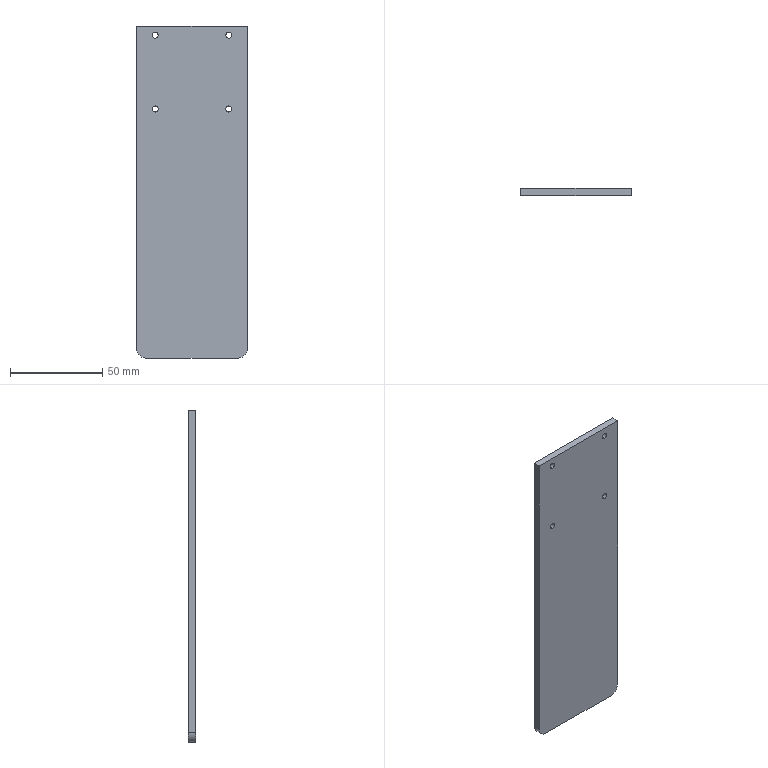Part | STEP file | PN_0021 Support plate | 1 solid | 16 faces | box 60 x 3.8 x 180 mm | volume 40869 mm3 | cylinder 10 | plane 6 | commonest cylinder face diameters 3.3 x8 10 x2
STEP:
#1=CARTESIAN_POINT('',(0.,0.,0.));
#2=DIRECTION('',(0.,0.,1.));
#3=DIRECTION('',(1.,0.,0.));
#4=AXIS2_PLACEMENT_3D('',#1,#2,#3);
#5=CARTESIAN_POINT('',(20.,0.,86.65));
#6=VERTEX_POINT('',#5);
#7=CARTESIAN_POINT('',(20.,3.8,86.65));
#8=VERTEX_POINT('',#7);
#9=CARTESIAN_POINT('',(20.,3.8,86.65));
#10=DIRECTION('',(0.,1.,0.));
#11=VECTOR('',#10,1.);
#12=LINE('',#9,#11);
#13=CARTESIAN_POINT('',(20.,3.8,85.));
#14=DIRECTION('',(0.,1.,0.));
#15=DIRECTION('',(0.,0.,1.));
#16=AXIS2_PLACEMENT_3D('',#13,#14,#15);
#17=CYLINDRICAL_SURFACE('',#16,1.65);
#18=CARTESIAN_POINT('',(6.283,0.));
#19=DIRECTION('',(0.,1.));
#20=VECTOR('',#19,1.);
#21=LINE('',#18,#20);
#22=(GEOMETRIC_REPRESENTATION_CONTEXT(2)PARAMETRIC_REPRESENTATION_CONTEXT()REPRESENTATION_CONTEXT('',''));
#23=DEFINITIONAL_REPRESENTATION('',(#21),#22);
#24=PCURVE('',#17,#23);
#25=CARTESIAN_POINT('',(20.,3.8,85.));
#26=DIRECTION('',(0.,1.,0.));
#27=DIRECTION('',(0.,0.,1.));
#28=AXIS2_PLACEMENT_3D('',#25,#26,#27);
#29=CYLINDRICAL_SURFACE('',#28,1.65);
#30=CARTESIAN_POINT('',(0.,0.));
#31=DIRECTION('',(0.,1.));
#32=VECTOR('',#31,1.);
#33=LINE('',#30,#32);
#34=(GEOMETRIC_REPRESENTATION_CONTEXT(2)PARAMETRIC_REPRESENTATION_CONTEXT()REPRESENTATION_CONTEXT('',''));
#35=DEFINITIONAL_REPRESENTATION('',(#33),#34);
#36=PCURVE('',#29,#35);
#37=SURFACE_CURVE('',#12,(#24,#36),.PCURVE_S1.);
#38=EDGE_CURVE('',#6,#8,#37,.T.);
#39=ORIENTED_EDGE('',*,*,#38,.T.);
#40=CARTESIAN_POINT('',(20.,3.8,83.35));
#41=VERTEX_POINT('',#40);
#42=CARTESIAN_POINT('',(20.,3.8,85.));
#43=DIRECTION('',(0.,-1.,0.));
#44=DIRECTION('',(0.,0.,1.));
#45=AXIS2_PLACEMENT_3D('',#42,#43,#44);
#46=CIRCLE('',#45,1.65);
#47=CARTESIAN_POINT('',(6.283,0.));
#48=DIRECTION('',(-1.,0.));
#49=VECTOR('',#48,1.);
#50=LINE('',#47,#49);
#51=(GEOMETRIC_REPRESENTATION_CONTEXT(2)PARAMETRIC_REPRESENTATION_CONTEXT()REPRESENTATION_CONTEXT('',''));
#52=DEFINITIONAL_REPRESENTATION('',(#50),#51);
#53=PCURVE('',#17,#52);
#54=CARTESIAN_POINT('',(0.,3.8,0.));
#55=DIRECTION('',(0.,1.,0.));
#56=DIRECTION('',(0.,0.,1.));
#57=AXIS2_PLACEMENT_3D('',#54,#55,#56);
#58=PLANE('',#57);
#59=CARTESIAN_POINT('',(86.65,20.));
#60=CARTESIAN_POINT('',(86.65,17.142));
#61=CARTESIAN_POINT('',(84.175,18.571));
#62=CARTESIAN_POINT('',(81.7,20.));
#63=CARTESIAN_POINT('',(84.175,21.429));
#64=CARTESIAN_POINT('',(86.65,22.858));
#65=CARTESIAN_POINT('',(86.65,20.));
#66=(BOUNDED_CURVE()B_SPLINE_CURVE(2,(#59,#60,#61,#62,#63,#64,#65),.UNSPECIFIED.,.T.,.F.)B_SPLINE_CURVE_WITH_KNOTS((1,2,2,2,2,1),(-2.094,0.,2.094,4.189,6.283,8.378),.UNSPECIFIED.)CURVE()GEOMETRIC_REPRESENTATION_ITEM()RATIONAL_B_SPLINE_CURVE((1.,0.5,1.,0.5,1.,0.5,1.))REPRESENTATION_ITEM(''));
#67=(GEOMETRIC_REPRESENTATION_CONTEXT(2)PARAMETRIC_REPRESENTATION_CONTEXT()REPRESENTATION_CONTEXT('',''));
#68=DEFINITIONAL_REPRESENTATION('',(#66),#67);
#69=PCURVE('',#58,#68);
#70=SURFACE_CURVE('',#46,(#53,#69),.PCURVE_S1.);
#71=EDGE_CURVE('',#8,#41,#70,.T.);
#72=ORIENTED_EDGE('',*,*,#71,.T.);
#73=CARTESIAN_POINT('',(20.,0.,83.35));
#74=VERTEX_POINT('',#73);
#75=CARTESIAN_POINT('',(20.,3.8,83.35));
#76=DIRECTION('',(0.,1.,0.));
#77=VECTOR('',#76,1.);
#78=LINE('',#75,#77);
#79=CARTESIAN_POINT('',(3.142,0.));
#80=DIRECTION('',(0.,1.));
#81=VECTOR('',#80,1.);
#82=LINE('',#79,#81);
#83=(GEOMETRIC_REPRESENTATION_CONTEXT(2)PARAMETRIC_REPRESENTATION_CONTEXT()REPRESENTATION_CONTEXT('',''));
#84=DEFINITIONAL_REPRESENTATION('',(#82),#83);
#85=PCURVE('',#17,#84);
#86=CARTESIAN_POINT('',(3.142,0.));
#87=DIRECTION('',(0.,1.));
#88=VECTOR('',#87,1.);
#89=LINE('',#86,#88);
#90=(GEOMETRIC_REPRESENTATION_CONTEXT(2)PARAMETRIC_REPRESENTATION_CONTEXT()REPRESENTATION_CONTEXT('',''));
#91=DEFINITIONAL_REPRESENTATION('',(#89),#90);
#92=PCURVE('',#29,#91);
#93=SURFACE_CURVE('',#78,(#85,#92),.PCURVE_S1.);
#94=EDGE_CURVE('',#74,#41,#93,.T.);
#95=ORIENTED_EDGE('',*,*,#94,.F.);
#96=CARTESIAN_POINT('',(20.,0.,85.));
#97=DIRECTION('',(0.,-1.,0.));
#98=DIRECTION('',(0.,0.,1.));
#99=AXIS2_PLACEMENT_3D('',#96,#97,#98);
#100=CIRCLE('',#99,1.65);
#101=CARTESIAN_POINT('',(6.283,-3.8));
#102=DIRECTION('',(-1.,0.));
#103=VECTOR('',#102,1.);
#104=LINE('',#101,#103);
#105=(GEOMETRIC_REPRESENTATION_CONTEXT(2)PARAMETRIC_REPRESENTATION_CONTEXT()REPRESENTATION_CONTEXT('',''));
#106=DEFINITIONAL_REPRESENTATION('',(#104),#105);
#107=PCURVE('',#17,#106);
#108=CARTESIAN_POINT('',(0.,0.,0.));
#109=DIRECTION('',(0.,1.,0.));
#110=DIRECTION('',(0.,0.,1.));
#111=AXIS2_PLACEMENT_3D('',#108,#109,#110);
#112=PLANE('',#111);
#113=CARTESIAN_POINT('',(86.65,20.));
#114=CARTESIAN_POINT('',(86.65,17.142));
#115=CARTESIAN_POINT('',(84.175,18.571));
#116=CARTESIAN_POINT('',(81.7,20.));
#117=CARTESIAN_POINT('',(84.175,21.429));
#118=CARTESIAN_POINT('',(86.65,22.858));
#119=CARTESIAN_POINT('',(86.65,20.));
#120=(BOUNDED_CURVE()B_SPLINE_CURVE(2,(#113,#114,#115,#116,#117,#118,#119),.UNSPECIFIED.,.T.,.F.)B_SPLINE_CURVE_WITH_KNOTS((1,2,2,2,2,1),(-2.094,0.,2.094,4.189,6.283,8.378),.UNSPECIFIED.)CURVE()GEOMETRIC_REPRESENTATION_ITEM()RATIONAL_B_SPLINE_CURVE((1.,0.5,1.,0.5,1.,0.5,1.))REPRESENTATION_ITEM(''));
#121=(GEOMETRIC_REPRESENTATION_CONTEXT(2)PARAMETRIC_REPRESENTATION_CONTEXT()REPRESENTATION_CONTEXT('',''));
#122=DEFINITIONAL_REPRESENTATION('',(#120),#121);
#123=PCURVE('',#112,#122);
#124=SURFACE_CURVE('',#100,(#107,#123),.PCURVE_S1.);
#125=EDGE_CURVE('',#6,#74,#124,.T.);
#126=ORIENTED_EDGE('',*,*,#125,.F.);
#127=EDGE_LOOP('',(#39,#72,#95,#126));
#128=FACE_BOUND('',#127,.F.);
#129=ADVANCED_FACE('',(#128),#17,.F.);
#130=CARTESIAN_POINT('',(20.,0.,46.65));
#131=VERTEX_POINT('',#130);
#132=CARTESIAN_POINT('',(20.,3.8,46.65));
#133=VERTEX_POINT('',#132);
#134=CARTESIAN_POINT('',(20.,3.8,46.65));
#135=DIRECTION('',(0.,1.,0.));
#136=VECTOR('',#135,1.);
#137=LINE('',#134,#136);
#138=CARTESIAN_POINT('',(20.,3.8,45.));
#139=DIRECTION('',(0.,1.,0.));
#140=DIRECTION('',(0.,0.,1.));
#141=AXIS2_PLACEMENT_3D('',#138,#139,#140);
#142=CYLINDRICAL_SURFACE('',#141,1.65);
#143=CARTESIAN_POINT('',(6.283,0.));
#144=DIRECTION('',(0.,1.));
#145=VECTOR('',#144,1.);
#146=LINE('',#143,#145);
#147=(GEOMETRIC_REPRESENTATION_CONTEXT(2)PARAMETRIC_REPRESENTATION_CONTEXT()REPRESENTATION_CONTEXT('',''));
#148=DEFINITIONAL_REPRESENTATION('',(#146),#147);
#149=PCURVE('',#142,#148);
#150=CARTESIAN_POINT('',(20.,3.8,45.));
#151=DIRECTION('',(0.,1.,0.));
#152=DIRECTION('',(0.,0.,1.));
#153=AXIS2_PLACEMENT_3D('',#150,#151,#152);
#154=CYLINDRICAL_SURFACE('',#153,1.65);
#155=CARTESIAN_POINT('',(0.,0.));
#156=DIRECTION('',(0.,1.));
#157=VECTOR('',#156,1.);
#158=LINE('',#155,#157);
#159=(GEOMETRIC_REPRESENTATION_CONTEXT(2)PARAMETRIC_REPRESENTATION_CONTEXT()REPRESENTATION_CONTEXT('',''));
#160=DEFINITIONAL_REPRESENTATION('',(#158),#159);
#161=PCURVE('',#154,#160);
#162=SURFACE_CURVE('',#137,(#149,#161),.PCURVE_S1.);
#163=EDGE_CURVE('',#131,#133,#162,.T.);
#164=ORIENTED_EDGE('',*,*,#163,.T.);
#165=CARTESIAN_POINT('',(20.,3.8,43.35));
#166=VERTEX_POINT('',#165);
#167=CARTESIAN_POINT('',(20.,3.8,45.));
#168=DIRECTION('',(0.,-1.,0.));
#169=DIRECTION('',(0.,0.,1.));
#170=AXIS2_PLACEMENT_3D('',#167,#168,#169);
#171=CIRCLE('',#170,1.65);
#172=CARTESIAN_POINT('',(6.283,0.));
#173=DIRECTION('',(-1.,0.));
#174=VECTOR('',#173,1.);
#175=LINE('',#172,#174);
#176=(GEOMETRIC_REPRESENTATION_CONTEXT(2)PARAMETRIC_REPRESENTATION_CONTEXT()REPRESENTATION_CONTEXT('',''));
#177=DEFINITIONAL_REPRESENTATION('',(#175),#176);
#178=PCURVE('',#142,#177);
#179=CARTESIAN_POINT('',(46.65,20.));
#180=CARTESIAN_POINT('',(46.65,17.142));
#181=CARTESIAN_POINT('',(44.175,18.571));
#182=CARTESIAN_POINT('',(41.7,20.));
#183=CARTESIAN_POINT('',(44.175,21.429));
#184=CARTESIAN_POINT('',(46.65,22.858));
#185=CARTESIAN_POINT('',(46.65,20.));
#186=(BOUNDED_CURVE()B_SPLINE_CURVE(2,(#179,#180,#181,#182,#183,#184,#185),.UNSPECIFIED.,.T.,.F.)B_SPLINE_CURVE_WITH_KNOTS((1,2,2,2,2,1),(-2.094,0.,2.094,4.189,6.283,8.378),.UNSPECIFIED.)CURVE()GEOMETRIC_REPRESENTATION_ITEM()RATIONAL_B_SPLINE_CURVE((1.,0.5,1.,0.5,1.,0.5,1.))REPRESENTATION_ITEM(''));
#187=(GEOMETRIC_REPRESENTATION_CONTEXT(2)PARAMETRIC_REPRESENTATION_CONTEXT()REPRESENTATION_CONTEXT('',''));
#188=DEFINITIONAL_REPRESENTATION('',(#186),#187);
#189=PCURVE('',#58,#188);
#190=SURFACE_CURVE('',#171,(#178,#189),.PCURVE_S1.);
#191=EDGE_CURVE('',#133,#166,#190,.T.);
#192=ORIENTED_EDGE('',*,*,#191,.T.);
#193=CARTESIAN_POINT('',(20.,0.,43.35));
#194=VERTEX_POINT('',#193);
#195=CARTESIAN_POINT('',(20.,3.8,43.35));
#196=DIRECTION('',(0.,1.,0.));
#197=VECTOR('',#196,1.);
#198=LINE('',#195,#197);
#199=CARTESIAN_POINT('',(3.142,0.));
#200=DIRECTION('',(0.,1.));
#201=VECTOR('',#200,1.);
#202=LINE('',#199,#201);
#203=(GEOMETRIC_REPRESENTATION_CONTEXT(2)PARAMETRIC_REPRESENTATION_CONTEXT()REPRESENTATION_CONTEXT('',''));
#204=DEFINITIONAL_REPRESENTATION('',(#202),#203);
#205=PCURVE('',#142,#204);
#206=CARTESIAN_POINT('',(3.142,0.));
#207=DIRECTION('',(0.,1.));
#208=VECTOR('',#207,1.);
#209=LINE('',#206,#208);
#210=(GEOMETRIC_REPRESENTATION_CONTEXT(2)PARAMETRIC_REPRESENTATION_CONTEXT()REPRESENTATION_CONTEXT('',''));
#211=DEFINITIONAL_REPRESENTATION('',(#209),#210);
#212=PCURVE('',#154,#211);
#213=SURFACE_CURVE('',#198,(#205,#212),.PCURVE_S1.);
#214=EDGE_CURVE('',#194,#166,#213,.T.);
#215=ORIENTED_EDGE('',*,*,#214,.F.);
#216=CARTESIAN_POINT('',(20.,0.,45.));
#217=DIRECTION('',(0.,-1.,0.));
#218=DIRECTION('',(0.,0.,1.));
#219=AXIS2_PLACEMENT_3D('',#216,#217,#218);
#220=CIRCLE('',#219,1.65);
#221=CARTESIAN_POINT('',(6.283,-3.8));
#222=DIRECTION('',(-1.,0.));
#223=VECTOR('',#222,1.);
#224=LINE('',#221,#223);
#225=(GEOMETRIC_REPRESENTATION_CONTEXT(2)PARAMETRIC_REPRESENTATION_CONTEXT()REPRESENTATION_CONTEXT('',''));
#226=DEFINITIONAL_REPRESENTATION('',(#224),#225);
#227=PCURVE('',#142,#226);
#228=CARTESIAN_POINT('',(46.65,20.));
#229=CARTESIAN_POINT('',(46.65,17.142));
#230=CARTESIAN_POINT('',(44.175,18.571));
#231=CARTESIAN_POINT('',(41.7,20.));
#232=CARTESIAN_POINT('',(44.175,21.429));
#233=CARTESIAN_POINT('',(46.65,22.858));
#234=CARTESIAN_POINT('',(46.65,20.));
#235=(BOUNDED_CURVE()B_SPLINE_CURVE(2,(#228,#229,#230,#231,#232,#233,#234),.UNSPECIFIED.,.T.,.F.)B_SPLINE_CURVE_WITH_KNOTS((1,2,2,2,2,1),(-2.094,0.,2.094,4.189,6.283,8.378),.UNSPECIFIED.)CURVE()GEOMETRIC_REPRESENTATION_ITEM()RATIONAL_B_SPLINE_CURVE((1.,0.5,1.,0.5,1.,0.5,1.))REPRESENTATION_ITEM(''));
#236=(GEOMETRIC_REPRESENTATION_CONTEXT(2)PARAMETRIC_REPRESENTATION_CONTEXT()REPRESENTATION_CONTEXT('',''));
#237=DEFINITIONAL_REPRESENTATION('',(#235),#236);
#238=PCURVE('',#112,#237);
#239=SURFACE_CURVE('',#220,(#227,#238),.PCURVE_S1.);
#240=EDGE_CURVE('',#131,#194,#239,.T.);
#241=ORIENTED_EDGE('',*,*,#240,.F.);
#242=EDGE_LOOP('',(#164,#192,#215,#241));
#243=FACE_BOUND('',#242,.F.);
#244=ADVANCED_FACE('',(#243),#142,.F.);
#245=CARTESIAN_POINT('',(-20.,0.,46.65));
#246=VERTEX_POINT('',#245);
#247=CARTESIAN_POINT('',(-20.,3.8,46.65));
#248=VERTEX_POINT('',#247);
#249=CARTESIAN_POINT('',(-20.,3.8,46.65));
#250=DIRECTION('',(0.,1.,0.));
#251=VECTOR('',#250,1.);
#252=LINE('',#249,#251);
#253=CARTESIAN_POINT('',(-20.,3.8,45.));
#254=DIRECTION('',(0.,1.,0.));
#255=DIRECTION('',(0.,0.,1.));
#256=AXIS2_PLACEMENT_3D('',#253,#254,#255);
#257=CYLINDRICAL_SURFACE('',#256,1.65);
#258=CARTESIAN_POINT('',(6.283,0.));
#259=DIRECTION('',(0.,1.));
#260=VECTOR('',#259,1.);
#261=LINE('',#258,#260);
#262=(GEOMETRIC_REPRESENTATION_CONTEXT(2)PARAMETRIC_REPRESENTATION_CONTEXT()REPRESENTATION_CONTEXT('',''));
#263=DEFINITIONAL_REPRESENTATION('',(#261),#262);
#264=PCURVE('',#257,#263);
#265=CARTESIAN_POINT('',(-20.,3.8,45.));
#266=DIRECTION('',(0.,1.,0.));
#267=DIRECTION('',(0.,0.,1.));
#268=AXIS2_PLACEMENT_3D('',#265,#266,#267);
#269=CYLINDRICAL_SURFACE('',#268,1.65);
#270=CARTESIAN_POINT('',(0.,0.));
#271=DIRECTION('',(0.,1.));
#272=VECTOR('',#271,1.);
#273=LINE('',#270,#272);
#274=(GEOMETRIC_REPRESENTATION_CONTEXT(2)PARAMETRIC_REPRESENTATION_CONTEXT()REPRESENTATION_CONTEXT('',''));
#275=DEFINITIONAL_REPRESENTATION('',(#273),#274);
#276=PCURVE('',#269,#275);
#277=SURFACE_CURVE('',#252,(#264,#276),.PCURVE_S1.);
#278=EDGE_CURVE('',#246,#248,#277,.T.);
#279=ORIENTED_EDGE('',*,*,#278,.T.);
#280=CARTESIAN_POINT('',(-20.,3.8,43.35));
#281=VERTEX_POINT('',#280);
#282=CARTESIAN_POINT('',(-20.,3.8,45.));
#283=DIRECTION('',(0.,-1.,0.));
#284=DIRECTION('',(0.,0.,1.));
#285=AXIS2_PLACEMENT_3D('',#282,#283,#284);
#286=CIRCLE('',#285,1.65);
#287=CARTESIAN_POINT('',(6.283,0.));
#288=DIRECTION('',(-1.,0.));
#289=VECTOR('',#288,1.);
#290=LINE('',#287,#289);
#291=(GEOMETRIC_REPRESENTATION_CONTEXT(2)PARAMETRIC_REPRESENTATION_CONTEXT()REPRESENTATION_CONTEXT('',''));
#292=DEFINITIONAL_REPRESENTATION('',(#290),#291);
#293=PCURVE('',#257,#292);
#294=CARTESIAN_POINT('',(46.65,-20.));
#295=CARTESIAN_POINT('',(46.65,-22.858));
#296=CARTESIAN_POINT('',(44.175,-21.429));
#297=CARTESIAN_POINT('',(41.7,-20.));
#298=CARTESIAN_POINT('',(44.175,-18.571));
#299=CARTESIAN_POINT('',(46.65,-17.142));
#300=CARTESIAN_POINT('',(46.65,-20.));
#301=(BOUNDED_CURVE()B_SPLINE_CURVE(2,(#294,#295,#296,#297,#298,#299,#300),.UNSPECIFIED.,.T.,.F.)B_SPLINE_CURVE_WITH_KNOTS((1,2,2,2,2,1),(-2.094,0.,2.094,4.189,6.283,8.378),.UNSPECIFIED.)CURVE()GEOMETRIC_REPRESENTATION_ITEM()RATIONAL_B_SPLINE_CURVE((1.,0.5,1.,0.5,1.,0.5,1.))REPRESENTATION_ITEM(''));
#302=(GEOMETRIC_REPRESENTATION_CONTEXT(2)PARAMETRIC_REPRESENTATION_CONTEXT()REPRESENTATION_CONTEXT('',''));
#303=DEFINITIONAL_REPRESENTATION('',(#301),#302);
#304=PCURVE('',#58,#303);
#305=SURFACE_CURVE('',#286,(#293,#304),.PCURVE_S1.);
#306=EDGE_CURVE('',#248,#281,#305,.T.);
#307=ORIENTED_EDGE('',*,*,#306,.T.);
#308=CARTESIAN_POINT('',(-20.,0.,43.35));
#309=VERTEX_POINT('',#308);
#310=CARTESIAN_POINT('',(-20.,3.8,43.35));
#311=DIRECTION('',(0.,1.,0.));
#312=VECTOR('',#311,1.);
#313=LINE('',#310,#312);
#314=CARTESIAN_POINT('',(3.142,0.));
#315=DIRECTION('',(0.,1.));
#316=VECTOR('',#315,1.);
#317=LINE('',#314,#316);
#318=(GEOMETRIC_REPRESENTATION_CONTEXT(2)PARAMETRIC_REPRESENTATION_CONTEXT()REPRESENTATION_CONTEXT('',''));
#319=DEFINITIONAL_REPRESENTATION('',(#317),#318);
#320=PCURVE('',#257,#319);
#321=CARTESIAN_POINT('',(3.142,0.));
#322=DIRECTION('',(0.,1.));
#323=VECTOR('',#322,1.);
#324=LINE('',#321,#323);
#325=(GEOMETRIC_REPRESENTATION_CONTEXT(2)PARAMETRIC_REPRESENTATION_CONTEXT()REPRESENTATION_CONTEXT('',''));
#326=DEFINITIONAL_REPRESENTATION('',(#324),#325);
#327=PCURVE('',#269,#326);
#328=SURFACE_CURVE('',#313,(#320,#327),.PCURVE_S1.);
#329=EDGE_CURVE('',#309,#281,#328,.T.);
#330=ORIENTED_EDGE('',*,*,#329,.F.);
#331=CARTESIAN_POINT('',(-20.,0.,45.));
#332=DIRECTION('',(0.,-1.,0.));
#333=DIRECTION('',(0.,0.,1.));
#334=AXIS2_PLACEMENT_3D('',#331,#332,#333);
#335=CIRCLE('',#334,1.65);
#336=CARTESIAN_POINT('',(6.283,-3.8));
#337=DIRECTION('',(-1.,0.));
#338=VECTOR('',#337,1.);
#339=LINE('',#336,#338);
#340=(GEOMETRIC_REPRESENTATION_CONTEXT(2)PARAMETRIC_REPRESENTATION_CONTEXT()REPRESENTATION_CONTEXT('',''));
#341=DEFINITIONAL_REPRESENTATION('',(#339),#340);
#342=PCURVE('',#257,#341);
#343=CARTESIAN_POINT('',(46.65,-20.));
#344=CARTESIAN_POINT('',(46.65,-22.858));
#345=CARTESIAN_POINT('',(44.175,-21.429));
#346=CARTESIAN_POINT('',(41.7,-20.));
#347=CARTESIAN_POINT('',(44.175,-18.571));
#348=CARTESIAN_POINT('',(46.65,-17.142));
#349=CARTESIAN_POINT('',(46.65,-20.));
#350=(BOUNDED_CURVE()B_SPLINE_CURVE(2,(#343,#344,#345,#346,#347,#348,#349),.UNSPECIFIED.,.T.,.F.)B_SPLINE_CURVE_WITH_KNOTS((1,2,2,2,2,1),(-2.094,0.,2.094,4.189,6.283,8.378),.UNSPECIFIED.)CURVE()GEOMETRIC_REPRESENTATION_ITEM()RATIONAL_B_SPLINE_CURVE((1.,0.5,1.,0.5,1.,0.5,1.))REPRESENTATION_ITEM(''));
#351=(GEOMETRIC_REPRESENTATION_CONTEXT(2)PARAMETRIC_REPRESENTATION_CONTEXT()REPRESENTATION_CONTEXT('',''));
#352=DEFINITIONAL_REPRESENTATION('',(#350),#351);
#353=PCURVE('',#112,#352);
#354=SURFACE_CURVE('',#335,(#342,#353),.PCURVE_S1.);
#355=EDGE_CURVE('',#246,#309,#354,.T.);
#356=ORIENTED_EDGE('',*,*,#355,.F.);
#357=EDGE_LOOP('',(#279,#307,#330,#356));
#358=FACE_BOUND('',#357,.F.);
#359=ADVANCED_FACE('',(#358),#257,.F.);
#360=CARTESIAN_POINT('',(-20.,0.,86.65));
#361=VERTEX_POINT('',#360);
#362=CARTESIAN_POINT('',(-20.,3.8,86.65));
#363=VERTEX_POINT('',#362);
#364=CARTESIAN_POINT('',(-20.,3.8,86.65));
#365=DIRECTION('',(0.,1.,0.));
#366=VECTOR('',#365,1.);
#367=LINE('',#364,#366);
#368=CARTESIAN_POINT('',(-20.,3.8,85.));
#369=DIRECTION('',(0.,1.,0.));
#370=DIRECTION('',(0.,0.,1.));
#371=AXIS2_PLACEMENT_3D('',#368,#369,#370);
#372=CYLINDRICAL_SURFACE('',#371,1.65);
#373=CARTESIAN_POINT('',(6.283,0.));
#374=DIRECTION('',(0.,1.));
#375=VECTOR('',#374,1.);
#376=LINE('',#373,#375);
#377=(GEOMETRIC_REPRESENTATION_CONTEXT(2)PARAMETRIC_REPRESENTATION_CONTEXT()REPRESENTATION_CONTEXT('',''));
#378=DEFINITIONAL_REPRESENTATION('',(#376),#377);
#379=PCURVE('',#372,#378);
#380=CARTESIAN_POINT('',(-20.,3.8,85.));
#381=DIRECTION('',(0.,1.,0.));
#382=DIRECTION('',(0.,0.,1.));
#383=AXIS2_PLACEMENT_3D('',#380,#381,#382);
#384=CYLINDRICAL_SURFACE('',#383,1.65);
#385=CARTESIAN_POINT('',(0.,0.));
#386=DIRECTION('',(0.,1.));
#387=VECTOR('',#386,1.);
#388=LINE('',#385,#387);
#389=(GEOMETRIC_REPRESENTATION_CONTEXT(2)PARAMETRIC_REPRESENTATION_CONTEXT()REPRESENTATION_CONTEXT('',''));
#390=DEFINITIONAL_REPRESENTATION('',(#388),#389);
#391=PCURVE('',#384,#390);
#392=SURFACE_CURVE('',#367,(#379,#391),.PCURVE_S1.);
#393=EDGE_CURVE('',#361,#363,#392,.T.);
#394=ORIENTED_EDGE('',*,*,#393,.T.);
#395=CARTESIAN_POINT('',(-20.,3.8,83.35));
#396=VERTEX_POINT('',#395);
#397=CARTESIAN_POINT('',(-20.,3.8,85.));
#398=DIRECTION('',(0.,-1.,0.));
#399=DIRECTION('',(0.,0.,1.));
#400=AXIS2_PLACEMENT_3D('',#397,#398,#399);
#401=CIRCLE('',#400,1.65);
#402=CARTESIAN_POINT('',(6.283,0.));
#403=DIRECTION('',(-1.,0.));
#404=VECTOR('',#403,1.);
#405=LINE('',#402,#404);
#406=(GEOMETRIC_REPRESENTATION_CONTEXT(2)PARAMETRIC_REPRESENTATION_CONTEXT()REPRESENTATION_CONTEXT('',''));
#407=DEFINITIONAL_REPRESENTATION('',(#405),#406);
#408=PCURVE('',#372,#407);
#409=CARTESIAN_POINT('',(86.65,-20.));
#410=CARTESIAN_POINT('',(86.65,-22.858));
#411=CARTESIAN_POINT('',(84.175,-21.429));
#412=CARTESIAN_POINT('',(81.7,-20.));
#413=CARTESIAN_POINT('',(84.175,-18.571));
#414=CARTESIAN_POINT('',(86.65,-17.142));
#415=CARTESIAN_POINT('',(86.65,-20.));
#416=(BOUNDED_CURVE()B_SPLINE_CURVE(2,(#409,#410,#411,#412,#413,#414,#415),.UNSPECIFIED.,.T.,.F.)B_SPLINE_CURVE_WITH_KNOTS((1,2,2,2,2,1),(-2.094,0.,2.094,4.189,6.283,8.378),.UNSPECIFIED.)CURVE()GEOMETRIC_REPRESENTATION_ITEM()RATIONAL_B_SPLINE_CURVE((1.,0.5,1.,0.5,1.,0.5,1.))REPRESENTATION_ITEM(''));
#417=(GEOMETRIC_REPRESENTATION_CONTEXT(2)PARAMETRIC_REPRESENTATION_CONTEXT()REPRESENTATION_CONTEXT('',''));
#418=DEFINITIONAL_REPRESENTATION('',(#416),#417);
#419=PCURVE('',#58,#418);
#420=SURFACE_CURVE('',#401,(#408,#419),.PCURVE_S1.);
#421=EDGE_CURVE('',#363,#396,#420,.T.);
#422=ORIENTED_EDGE('',*,*,#421,.T.);
#423=CARTESIAN_POINT('',(-20.,0.,83.35));
#424=VERTEX_POINT('',#423);
#425=CARTESIAN_POINT('',(-20.,3.8,83.35));
#426=DIRECTION('',(0.,1.,0.));
#427=VECTOR('',#426,1.);
#428=LINE('',#425,#427);
#429=CARTESIAN_POINT('',(3.142,0.));
#430=DIRECTION('',(0.,1.));
#431=VECTOR('',#430,1.);
#432=LINE('',#429,#431);
#433=(GEOMETRIC_REPRESENTATION_CONTEXT(2)PARAMETRIC_REPRESENTATION_CONTEXT()REPRESENTATION_CONTEXT('',''));
#434=DEFINITIONAL_REPRESENTATION('',(#432),#433);
#435=PCURVE('',#372,#434);
#436=CARTESIAN_POINT('',(3.142,0.));
#437=DIRECTION('',(0.,1.));
#438=VECTOR('',#437,1.);
#439=LINE('',#436,#438);
#440=(GEOMETRIC_REPRESENTATION_CONTEXT(2)PARAMETRIC_REPRESENTATION_CONTEXT()REPRESENTATION_CONTEXT('',''));
#441=DEFINITIONAL_REPRESENTATION('',(#439),#440);
#442=PCURVE('',#384,#441);
#443=SURFACE_CURVE('',#428,(#435,#442),.PCURVE_S1.);
#444=EDGE_CURVE('',#424,#396,#443,.T.);
#445=ORIENTED_EDGE('',*,*,#444,.F.);
#446=CARTESIAN_POINT('',(-20.,0.,85.));
#447=DIRECTION('',(0.,-1.,0.));
#448=DIRECTION('',(0.,0.,1.));
#449=AXIS2_PLACEMENT_3D('',#446,#447,#448);
#450=CIRCLE('',#449,1.65);
#451=CARTESIAN_POINT('',(6.283,-3.8));
#452=DIRECTION('',(-1.,0.));
#453=VECTOR('',#452,1.);
#454=LINE('',#451,#453);
#455=(GEOMETRIC_REPRESENTATION_CONTEXT(2)PARAMETRIC_REPRESENTATION_CONTEXT()REPRESENTATION_CONTEXT('',''));
#456=DEFINITIONAL_REPRESENTATION('',(#454),#455);
#457=PCURVE('',#372,#456);
#458=CARTESIAN_POINT('',(86.65,-20.));
#459=CARTESIAN_POINT('',(86.65,-22.858));
#460=CARTESIAN_POINT('',(84.175,-21.429));
#461=CARTESIAN_POINT('',(81.7,-20.));
#462=CARTESIAN_POINT('',(84.175,-18.571));
#463=CARTESIAN_POINT('',(86.65,-17.142));
#464=CARTESIAN_POINT('',(86.65,-20.));
#465=(BOUNDED_CURVE()B_SPLINE_CURVE(2,(#458,#459,#460,#461,#462,#463,#464),.UNSPECIFIED.,.T.,.F.)B_SPLINE_CURVE_WITH_KNOTS((1,2,2,2,2,1),(-2.094,0.,2.094,4.189,6.283,8.378),.UNSPECIFIED.)CURVE()GEOMETRIC_REPRESENTATION_ITEM()RATIONAL_B_SPLINE_CURVE((1.,0.5,1.,0.5,1.,0.5,1.))REPRESENTATION_ITEM(''));
#466=(GEOMETRIC_REPRESENTATION_CONTEXT(2)PARAMETRIC_REPRESENTATION_CONTEXT()REPRESENTATION_CONTEXT('',''));
#467=DEFINITIONAL_REPRESENTATION('',(#465),#466);
#468=PCURVE('',#112,#467);
#469=SURFACE_CURVE('',#450,(#457,#468),.PCURVE_S1.);
#470=EDGE_CURVE('',#361,#424,#469,.T.);
#471=ORIENTED_EDGE('',*,*,#470,.F.);
#472=EDGE_LOOP('',(#394,#422,#445,#471));
#473=FACE_BOUND('',#472,.F.);
#474=ADVANCED_FACE('',(#473),#372,.F.);
#475=CARTESIAN_POINT('',(-25.,0.,-90.));
#476=VERTEX_POINT('',#475);
#477=CARTESIAN_POINT('',(-30.,0.,-85.));
#478=VERTEX_POINT('',#477);
#479=CARTESIAN_POINT('',(-25.,0.,-85.));
#480=DIRECTION('',(0.,1.,0.));
#481=DIRECTION('',(0.,0.,-1.));
#482=AXIS2_PLACEMENT_3D('',#479,#480,#481);
#483=CIRCLE('',#482,5.);
#484=CARTESIAN_POINT('',(-85.,-25.));
#485=DIRECTION('',(-1.,0.));
#486=AXIS2_PLACEMENT_2D('',#484,#485);
#487=CIRCLE('',#486,5.);
#488=(GEOMETRIC_REPRESENTATION_CONTEXT(2)PARAMETRIC_REPRESENTATION_CONTEXT()REPRESENTATION_CONTEXT('',''));
#489=DEFINITIONAL_REPRESENTATION('',(#487),#488);
#490=PCURVE('',#112,#489);
#491=CARTESIAN_POINT('',(-25.,3.8,-85.));
#492=DIRECTION('',(0.,-1.,0.));
#493=DIRECTION('',(0.,0.,-1.));
#494=AXIS2_PLACEMENT_3D('',#491,#492,#493);
#495=CYLINDRICAL_SURFACE('',#494,5.);
#496=CARTESIAN_POINT('',(6.283,3.8));
#497=DIRECTION('',(-1.,0.));
#498=VECTOR('',#497,1.);
#499=LINE('',#496,#498);
#500=(GEOMETRIC_REPRESENTATION_CONTEXT(2)PARAMETRIC_REPRESENTATION_CONTEXT()REPRESENTATION_CONTEXT('',''));
#501=DEFINITIONAL_REPRESENTATION('',(#499),#500);
#502=PCURVE('',#495,#501);
#503=SURFACE_CURVE('',#483,(#490,#502),.PCURVE_S1.);
#504=EDGE_CURVE('',#476,#478,#503,.T.);
#505=ORIENTED_EDGE('',*,*,#504,.F.);
#506=CARTESIAN_POINT('',(25.,0.,-90.));
#507=VERTEX_POINT('',#506);
#508=CARTESIAN_POINT('',(0.,0.,-90.));
#509=DIRECTION('',(-1.,0.,0.));
#510=VECTOR('',#509,1.);
#511=LINE('',#508,#510);
#512=CARTESIAN_POINT('',(-90.,0.));
#513=DIRECTION('',(0.,-1.));
#514=VECTOR('',#513,1.);
#515=LINE('',#512,#514);
#516=(GEOMETRIC_REPRESENTATION_CONTEXT(2)PARAMETRIC_REPRESENTATION_CONTEXT()REPRESENTATION_CONTEXT('',''));
#517=DEFINITIONAL_REPRESENTATION('',(#515),#516);
#518=PCURVE('',#112,#517);
#519=CARTESIAN_POINT('',(-30.,3.8,-90.));
#520=DIRECTION('',(0.,0.,1.));
#521=DIRECTION('',(1.,0.,0.));
#522=AXIS2_PLACEMENT_3D('',#519,#520,#521);
#523=PLANE('',#522);
#524=CARTESIAN_POINT('',(30.,-3.8));
#525=DIRECTION('',(-1.,0.));
#526=VECTOR('',#525,1.);
#527=LINE('',#524,#526);
#528=(GEOMETRIC_REPRESENTATION_CONTEXT(2)PARAMETRIC_REPRESENTATION_CONTEXT()REPRESENTATION_CONTEXT('',''));
#529=DEFINITIONAL_REPRESENTATION('',(#527),#528);
#530=PCURVE('',#523,#529);
#531=SURFACE_CURVE('',#511,(#518,#530),.PCURVE_S1.);
#532=EDGE_CURVE('',#507,#476,#531,.T.);
#533=ORIENTED_EDGE('',*,*,#532,.F.);
#534=CARTESIAN_POINT('',(30.,0.,-85.));
#535=VERTEX_POINT('',#534);
#536=CARTESIAN_POINT('',(25.,0.,-85.));
#537=DIRECTION('',(0.,1.,0.));
#538=DIRECTION('',(0.,0.,-1.));
#539=AXIS2_PLACEMENT_3D('',#536,#537,#538);
#540=CIRCLE('',#539,5.);
#541=CARTESIAN_POINT('',(-85.,25.));
#542=DIRECTION('',(-1.,0.));
#543=AXIS2_PLACEMENT_2D('',#541,#542);
#544=CIRCLE('',#543,5.);
#545=(GEOMETRIC_REPRESENTATION_CONTEXT(2)PARAMETRIC_REPRESENTATION_CONTEXT()REPRESENTATION_CONTEXT('',''));
#546=DEFINITIONAL_REPRESENTATION('',(#544),#545);
#547=PCURVE('',#112,#546);
#548=CARTESIAN_POINT('',(25.,3.8,-85.));
#549=DIRECTION('',(0.,-1.,0.));
#550=DIRECTION('',(0.,0.,-1.));
#551=AXIS2_PLACEMENT_3D('',#548,#549,#550);
#552=CYLINDRICAL_SURFACE('',#551,5.);
#553=CARTESIAN_POINT('',(6.283,3.8));
#554=DIRECTION('',(-1.,0.));
#555=VECTOR('',#554,1.);
#556=LINE('',#553,#555);
#557=(GEOMETRIC_REPRESENTATION_CONTEXT(2)PARAMETRIC_REPRESENTATION_CONTEXT()REPRESENTATION_CONTEXT('',''));
#558=DEFINITIONAL_REPRESENTATION('',(#556),#557);
#559=PCURVE('',#552,#558);
#560=SURFACE_CURVE('',#540,(#547,#559),.PCURVE_S1.);
#561=EDGE_CURVE('',#535,#507,#560,.T.);
#562=ORIENTED_EDGE('',*,*,#561,.F.);
#563=CARTESIAN_POINT('',(30.,0.,90.));
#564=VERTEX_POINT('',#563);
#565=CARTESIAN_POINT('',(30.,0.,0.));
#566=DIRECTION('',(0.,0.,-1.));
#567=VECTOR('',#566,1.);
#568=LINE('',#565,#567);
#569=CARTESIAN_POINT('',(0.,30.));
#570=DIRECTION('',(-1.,0.));
#571=VECTOR('',#570,1.);
#572=LINE('',#569,#571);
#573=(GEOMETRIC_REPRESENTATION_CONTEXT(2)PARAMETRIC_REPRESENTATION_CONTEXT()REPRESENTATION_CONTEXT('',''));
#574=DEFINITIONAL_REPRESENTATION('',(#572),#573);
#575=PCURVE('',#112,#574);
#576=CARTESIAN_POINT('',(30.,3.8,-90.));
#577=DIRECTION('',(-1.,0.,0.));
#578=DIRECTION('',(0.,0.,1.));
#579=AXIS2_PLACEMENT_3D('',#576,#577,#578);
#580=PLANE('',#579);
#581=CARTESIAN_POINT('',(90.,-3.8));
#582=DIRECTION('',(-1.,0.));
#583=VECTOR('',#582,1.);
#584=LINE('',#581,#583);
#585=(GEOMETRIC_REPRESENTATION_CONTEXT(2)PARAMETRIC_REPRESENTATION_CONTEXT()REPRESENTATION_CONTEXT('',''));
#586=DEFINITIONAL_REPRESENTATION('',(#584),#585);
#587=PCURVE('',#580,#586);
#588=SURFACE_CURVE('',#568,(#575,#587),.PCURVE_S1.);
#589=EDGE_CURVE('',#564,#535,#588,.T.);
#590=ORIENTED_EDGE('',*,*,#589,.F.);
#591=CARTESIAN_POINT('',(-30.,0.,90.));
#592=VERTEX_POINT('',#591);
#593=CARTESIAN_POINT('',(0.,0.,90.));
#594=DIRECTION('',(1.,0.,0.));
#595=VECTOR('',#594,1.);
#596=LINE('',#593,#595);
#597=CARTESIAN_POINT('',(90.,0.));
#598=DIRECTION('',(0.,1.));
#599=VECTOR('',#598,1.);
#600=LINE('',#597,#599);
#601=(GEOMETRIC_REPRESENTATION_CONTEXT(2)PARAMETRIC_REPRESENTATION_CONTEXT()REPRESENTATION_CONTEXT('',''));
#602=DEFINITIONAL_REPRESENTATION('',(#600),#601);
#603=PCURVE('',#112,#602);
#604=CARTESIAN_POINT('',(-30.,3.8,90.));
#605=DIRECTION('',(0.,0.,-1.));
#606=DIRECTION('',(-1.,0.,0.));
#607=AXIS2_PLACEMENT_3D('',#604,#605,#606);
#608=PLANE('',#607);
#609=CARTESIAN_POINT('',(-30.,-3.8));
#610=DIRECTION('',(-1.,0.));
#611=VECTOR('',#610,1.);
#612=LINE('',#609,#611);
#613=(GEOMETRIC_REPRESENTATION_CONTEXT(2)PARAMETRIC_REPRESENTATION_CONTEXT()REPRESENTATION_CONTEXT('',''));
#614=DEFINITIONAL_REPRESENTATION('',(#612),#613);
#615=PCURVE('',#608,#614);
#616=SURFACE_CURVE('',#596,(#603,#615),.PCURVE_S1.);
#617=EDGE_CURVE('',#592,#564,#616,.T.);
#618=ORIENTED_EDGE('',*,*,#617,.F.);
#619=CARTESIAN_POINT('',(-30.,0.,0.));
#620=DIRECTION('',(0.,0.,1.));
#621=VECTOR('',#620,1.);
#622=LINE('',#619,#621);
#623=CARTESIAN_POINT('',(0.,-30.));
#624=DIRECTION('',(1.,0.));
#625=VECTOR('',#624,1.);
#626=LINE('',#623,#625);
#627=(GEOMETRIC_REPRESENTATION_CONTEXT(2)PARAMETRIC_REPRESENTATION_CONTEXT()REPRESENTATION_CONTEXT('',''));
#628=DEFINITIONAL_REPRESENTATION('',(#626),#627);
#629=PCURVE('',#112,#628);
#630=CARTESIAN_POINT('',(-30.,3.8,-90.));
#631=DIRECTION('',(1.,0.,0.));
#632=DIRECTION('',(0.,0.,-1.));
#633=AXIS2_PLACEMENT_3D('',#630,#631,#632);
#634=PLANE('',#633);
#635=CARTESIAN_POINT('',(-90.,-3.8));
#636=DIRECTION('',(-1.,0.));
#637=VECTOR('',#636,1.);
#638=LINE('',#635,#637);
#639=(GEOMETRIC_REPRESENTATION_CONTEXT(2)PARAMETRIC_REPRESENTATION_CONTEXT()REPRESENTATION_CONTEXT('',''));
#640=DEFINITIONAL_REPRESENTATION('',(#638),#639);
#641=PCURVE('',#634,#640);
#642=SURFACE_CURVE('',#622,(#629,#641),.PCURVE_S1.);
#643=EDGE_CURVE('',#478,#592,#642,.T.);
#644=ORIENTED_EDGE('',*,*,#643,.F.);
#645=EDGE_LOOP('',(#505,#533,#562,#590,#618,#644));
#646=FACE_BOUND('',#645,.T.);
#647=ORIENTED_EDGE('',*,*,#125,.F.);
#648=CARTESIAN_POINT('',(20.,0.,85.));
#649=DIRECTION('',(0.,-1.,0.));
#650=DIRECTION('',(0.,0.,1.));
#651=AXIS2_PLACEMENT_3D('',#648,#649,#650);
#652=CIRCLE('',#651,1.65);
#653=CARTESIAN_POINT('',(86.65,20.));
#654=CARTESIAN_POINT('',(86.65,17.142));
#655=CARTESIAN_POINT('',(84.175,18.571));
#656=CARTESIAN_POINT('',(81.7,20.));
#657=CARTESIAN_POINT('',(84.175,21.429));
#658=CARTESIAN_POINT('',(86.65,22.858));
#659=CARTESIAN_POINT('',(86.65,20.));
#660=(BOUNDED_CURVE()B_SPLINE_CURVE(2,(#653,#654,#655,#656,#657,#658,#659),.UNSPECIFIED.,.T.,.F.)B_SPLINE_CURVE_WITH_KNOTS((1,2,2,2,2,1),(-2.094,0.,2.094,4.189,6.283,8.378),.UNSPECIFIED.)CURVE()GEOMETRIC_REPRESENTATION_ITEM()RATIONAL_B_SPLINE_CURVE((1.,0.5,1.,0.5,1.,0.5,1.))REPRESENTATION_ITEM(''));
#661=(GEOMETRIC_REPRESENTATION_CONTEXT(2)PARAMETRIC_REPRESENTATION_CONTEXT()REPRESENTATION_CONTEXT('',''));
#662=DEFINITIONAL_REPRESENTATION('',(#660),#661);
#663=PCURVE('',#112,#662);
#664=CARTESIAN_POINT('',(6.283,-3.8));
#665=DIRECTION('',(-1.,0.));
#666=VECTOR('',#665,1.);
#667=LINE('',#664,#666);
#668=(GEOMETRIC_REPRESENTATION_CONTEXT(2)PARAMETRIC_REPRESENTATION_CONTEXT()REPRESENTATION_CONTEXT('',''));
#669=DEFINITIONAL_REPRESENTATION('',(#667),#668);
#670=PCURVE('',#29,#669);
#671=SURFACE_CURVE('',#652,(#663,#670),.PCURVE_S1.);
#672=EDGE_CURVE('',#74,#6,#671,.T.);
#673=ORIENTED_EDGE('',*,*,#672,.F.);
#674=EDGE_LOOP('',(#647,#673));
#675=FACE_BOUND('',#674,.T.);
#676=ORIENTED_EDGE('',*,*,#240,.F.);
#677=CARTESIAN_POINT('',(20.,0.,45.));
#678=DIRECTION('',(0.,-1.,0.));
#679=DIRECTION('',(0.,0.,1.));
#680=AXIS2_PLACEMENT_3D('',#677,#678,#679);
#681=CIRCLE('',#680,1.65);
#682=CARTESIAN_POINT('',(46.65,20.));
#683=CARTESIAN_POINT('',(46.65,17.142));
#684=CARTESIAN_POINT('',(44.175,18.571));
#685=CARTESIAN_POINT('',(41.7,20.));
#686=CARTESIAN_POINT('',(44.175,21.429));
#687=CARTESIAN_POINT('',(46.65,22.858));
#688=CARTESIAN_POINT('',(46.65,20.));
#689=(BOUNDED_CURVE()B_SPLINE_CURVE(2,(#682,#683,#684,#685,#686,#687,#688),.UNSPECIFIED.,.T.,.F.)B_SPLINE_CURVE_WITH_KNOTS((1,2,2,2,2,1),(-2.094,0.,2.094,4.189,6.283,8.378),.UNSPECIFIED.)CURVE()GEOMETRIC_REPRESENTATION_ITEM()RATIONAL_B_SPLINE_CURVE((1.,0.5,1.,0.5,1.,0.5,1.))REPRESENTATION_ITEM(''));
#690=(GEOMETRIC_REPRESENTATION_CONTEXT(2)PARAMETRIC_REPRESENTATION_CONTEXT()REPRESENTATION_CONTEXT('',''));
#691=DEFINITIONAL_REPRESENTATION('',(#689),#690);
#692=PCURVE('',#112,#691);
#693=CARTESIAN_POINT('',(6.283,-3.8));
#694=DIRECTION('',(-1.,0.));
#695=VECTOR('',#694,1.);
#696=LINE('',#693,#695);
#697=(GEOMETRIC_REPRESENTATION_CONTEXT(2)PARAMETRIC_REPRESENTATION_CONTEXT()REPRESENTATION_CONTEXT('',''));
#698=DEFINITIONAL_REPRESENTATION('',(#696),#697);
#699=PCURVE('',#154,#698);
#700=SURFACE_CURVE('',#681,(#692,#699),.PCURVE_S1.);
#701=EDGE_CURVE('',#194,#131,#700,.T.);
#702=ORIENTED_EDGE('',*,*,#701,.F.);
#703=EDGE_LOOP('',(#676,#702));
#704=FACE_BOUND('',#703,.T.);
#705=ORIENTED_EDGE('',*,*,#355,.F.);
#706=CARTESIAN_POINT('',(-20.,0.,45.));
#707=DIRECTION('',(0.,-1.,0.));
#708=DIRECTION('',(0.,0.,1.));
#709=AXIS2_PLACEMENT_3D('',#706,#707,#708);
#710=CIRCLE('',#709,1.65);
#711=CARTESIAN_POINT('',(46.65,-20.));
#712=CARTESIAN_POINT('',(46.65,-22.858));
#713=CARTESIAN_POINT('',(44.175,-21.429));
#714=CARTESIAN_POINT('',(41.7,-20.));
#715=CARTESIAN_POINT('',(44.175,-18.571));
#716=CARTESIAN_POINT('',(46.65,-17.142));
#717=CARTESIAN_POINT('',(46.65,-20.));
#718=(BOUNDED_CURVE()B_SPLINE_CURVE(2,(#711,#712,#713,#714,#715,#716,#717),.UNSPECIFIED.,.T.,.F.)B_SPLINE_CURVE_WITH_KNOTS((1,2,2,2,2,1),(-2.094,0.,2.094,4.189,6.283,8.378),.UNSPECIFIED.)CURVE()GEOMETRIC_REPRESENTATION_ITEM()RATIONAL_B_SPLINE_CURVE((1.,0.5,1.,0.5,1.,0.5,1.))REPRESENTATION_ITEM(''));
#719=(GEOMETRIC_REPRESENTATION_CONTEXT(2)PARAMETRIC_REPRESENTATION_CONTEXT()REPRESENTATION_CONTEXT('',''));
#720=DEFINITIONAL_REPRESENTATION('',(#718),#719);
#721=PCURVE('',#112,#720);
#722=CARTESIAN_POINT('',(6.283,-3.8));
#723=DIRECTION('',(-1.,0.));
#724=VECTOR('',#723,1.);
#725=LINE('',#722,#724);
#726=(GEOMETRIC_REPRESENTATION_CONTEXT(2)PARAMETRIC_REPRESENTATION_CONTEXT()REPRESENTATION_CONTEXT('',''));
#727=DEFINITIONAL_REPRESENTATION('',(#725),#726);
#728=PCURVE('',#269,#727);
#729=SURFACE_CURVE('',#710,(#721,#728),.PCURVE_S1.);
#730=EDGE_CURVE('',#309,#246,#729,.T.);
#731=ORIENTED_EDGE('',*,*,#730,.F.);
#732=EDGE_LOOP('',(#705,#731));
#733=FACE_BOUND('',#732,.T.);
#734=ORIENTED_EDGE('',*,*,#470,.F.);
#735=CARTESIAN_POINT('',(-20.,0.,85.));
#736=DIRECTION('',(0.,-1.,0.));
#737=DIRECTION('',(0.,0.,1.));
#738=AXIS2_PLACEMENT_3D('',#735,#736,#737);
#739=CIRCLE('',#738,1.65);
#740=CARTESIAN_POINT('',(86.65,-20.));
#741=CARTESIAN_POINT('',(86.65,-22.858));
#742=CARTESIAN_POINT('',(84.175,-21.429));
#743=CARTESIAN_POINT('',(81.7,-20.));
#744=CARTESIAN_POINT('',(84.175,-18.571));
#745=CARTESIAN_POINT('',(86.65,-17.142));
#746=CARTESIAN_POINT('',(86.65,-20.));
#747=(BOUNDED_CURVE()B_SPLINE_CURVE(2,(#740,#741,#742,#743,#744,#745,#746),.UNSPECIFIED.,.T.,.F.)B_SPLINE_CURVE_WITH_KNOTS((1,2,2,2,2,1),(-2.094,0.,2.094,4.189,6.283,8.378),.UNSPECIFIED.)CURVE()GEOMETRIC_REPRESENTATION_ITEM()RATIONAL_B_SPLINE_CURVE((1.,0.5,1.,0.5,1.,0.5,1.))REPRESENTATION_ITEM(''));
#748=(GEOMETRIC_REPRESENTATION_CONTEXT(2)PARAMETRIC_REPRESENTATION_CONTEXT()REPRESENTATION_CONTEXT('',''));
#749=DEFINITIONAL_REPRESENTATION('',(#747),#748);
#750=PCURVE('',#112,#749);
#751=CARTESIAN_POINT('',(6.283,-3.8));
#752=DIRECTION('',(-1.,0.));
#753=VECTOR('',#752,1.);
#754=LINE('',#751,#753);
#755=(GEOMETRIC_REPRESENTATION_CONTEXT(2)PARAMETRIC_REPRESENTATION_CONTEXT()REPRESENTATION_CONTEXT('',''));
#756=DEFINITIONAL_REPRESENTATION('',(#754),#755);
#757=PCURVE('',#384,#756);
#758=SURFACE_CURVE('',#739,(#750,#757),.PCURVE_S1.);
#759=EDGE_CURVE('',#424,#361,#758,.T.);
#760=ORIENTED_EDGE('',*,*,#759,.F.);
#761=EDGE_LOOP('',(#734,#760));
#762=FACE_BOUND('',#761,.T.);
#763=ADVANCED_FACE('',(#646,#675,#704,#733,#762),#112,.F.);
#764=CARTESIAN_POINT('',(-30.,3.8,-85.));
#765=VERTEX_POINT('',#764);
#766=CARTESIAN_POINT('',(-30.,3.8,-85.));
#767=DIRECTION('',(0.,1.,0.));
#768=VECTOR('',#767,1.);
#769=LINE('',#766,#768);
#770=CARTESIAN_POINT('',(-5.,0.));
#771=DIRECTION('',(0.,1.));
#772=VECTOR('',#771,1.);
#773=LINE('',#770,#772);
#774=(GEOMETRIC_REPRESENTATION_CONTEXT(2)PARAMETRIC_REPRESENTATION_CONTEXT()REPRESENTATION_CONTEXT('',''));
#775=DEFINITIONAL_REPRESENTATION('',(#773),#774);
#776=PCURVE('',#634,#775);
#777=CARTESIAN_POINT('',(4.712,0.));
#778=DIRECTION('',(0.,-1.));
#779=VECTOR('',#778,1.);
#780=LINE('',#777,#779);
#781=(GEOMETRIC_REPRESENTATION_CONTEXT(2)PARAMETRIC_REPRESENTATION_CONTEXT()REPRESENTATION_CONTEXT('',''));
#782=DEFINITIONAL_REPRESENTATION('',(#780),#781);
#783=PCURVE('',#495,#782);
#784=SURFACE_CURVE('',#769,(#776,#783),.PCURVE_S1.);
#785=EDGE_CURVE('',#478,#765,#784,.T.);
#786=ORIENTED_EDGE('',*,*,#785,.F.);
#787=ORIENTED_EDGE('',*,*,#643,.T.);
#788=CARTESIAN_POINT('',(-30.,3.8,90.));
#789=VERTEX_POINT('',#788);
#790=CARTESIAN_POINT('',(-30.,3.8,90.));
#791=DIRECTION('',(0.,-1.,0.));
#792=VECTOR('',#791,1.);
#793=LINE('',#790,#792);
#794=CARTESIAN_POINT('',(-180.,0.));
#795=DIRECTION('',(0.,-1.));
#796=VECTOR('',#795,1.);
#797=LINE('',#794,#796);
#798=(GEOMETRIC_REPRESENTATION_CONTEXT(2)PARAMETRIC_REPRESENTATION_CONTEXT()REPRESENTATION_CONTEXT('',''));
#799=DEFINITIONAL_REPRESENTATION('',(#797),#798);
#800=PCURVE('',#634,#799);
#801=CARTESIAN_POINT('',(0.,0.));
#802=DIRECTION('',(0.,-1.));
#803=VECTOR('',#802,1.);
#804=LINE('',#801,#803);
#805=(GEOMETRIC_REPRESENTATION_CONTEXT(2)PARAMETRIC_REPRESENTATION_CONTEXT()REPRESENTATION_CONTEXT('',''));
#806=DEFINITIONAL_REPRESENTATION('',(#804),#805);
#807=PCURVE('',#608,#806);
#808=SURFACE_CURVE('',#793,(#800,#807),.PCURVE_S1.);
#809=EDGE_CURVE('',#789,#592,#808,.T.);
#810=ORIENTED_EDGE('',*,*,#809,.F.);
#811=CARTESIAN_POINT('',(-30.,3.8,-90.));
#812=DIRECTION('',(0.,0.,1.));
#813=VECTOR('',#812,1.);
#814=LINE('',#811,#813);
#815=CARTESIAN_POINT('',(0.,0.));
#816=DIRECTION('',(-1.,0.));
#817=VECTOR('',#816,1.);
#818=LINE('',#815,#817);
#819=(GEOMETRIC_REPRESENTATION_CONTEXT(2)PARAMETRIC_REPRESENTATION_CONTEXT()REPRESENTATION_CONTEXT('',''));
#820=DEFINITIONAL_REPRESENTATION('',(#818),#819);
#821=PCURVE('',#634,#820);
#822=CARTESIAN_POINT('',(-90.,-30.));
#823=DIRECTION('',(1.,0.));
#824=VECTOR('',#823,1.);
#825=LINE('',#822,#824);
#826=(GEOMETRIC_REPRESENTATION_CONTEXT(2)PARAMETRIC_REPRESENTATION_CONTEXT()REPRESENTATION_CONTEXT('',''));
#827=DEFINITIONAL_REPRESENTATION('',(#825),#826);
#828=PCURVE('',#58,#827);
#829=SURFACE_CURVE('',#814,(#821,#828),.PCURVE_S1.);
#830=EDGE_CURVE('',#765,#789,#829,.T.);
#831=ORIENTED_EDGE('',*,*,#830,.F.);
#832=EDGE_LOOP('',(#786,#787,#810,#831));
#833=FACE_BOUND('',#832,.T.);
#834=ADVANCED_FACE('',(#833),#634,.F.);
#835=ORIENTED_EDGE('',*,*,#504,.T.);
#836=ORIENTED_EDGE('',*,*,#785,.T.);
#837=CARTESIAN_POINT('',(-25.,3.8,-90.));
#838=VERTEX_POINT('',#837);
#839=CARTESIAN_POINT('',(-25.,3.8,-85.));
#840=DIRECTION('',(0.,-1.,0.));
#841=DIRECTION('',(0.,0.,-1.));
#842=AXIS2_PLACEMENT_3D('',#839,#840,#841);
#843=CIRCLE('',#842,5.);
#844=CARTESIAN_POINT('',(0.,0.));
#845=DIRECTION('',(1.,0.));
#846=VECTOR('',#845,1.);
#847=LINE('',#844,#846);
#848=(GEOMETRIC_REPRESENTATION_CONTEXT(2)PARAMETRIC_REPRESENTATION_CONTEXT()REPRESENTATION_CONTEXT('',''));
#849=DEFINITIONAL_REPRESENTATION('',(#847),#848);
#850=PCURVE('',#495,#849);
#851=CARTESIAN_POINT('',(-90.,-25.));
#852=CARTESIAN_POINT('',(-90.,-16.34));
#853=CARTESIAN_POINT('',(-82.5,-20.67));
#854=CARTESIAN_POINT('',(-75.,-25.));
#855=CARTESIAN_POINT('',(-82.5,-29.33));
#856=CARTESIAN_POINT('',(-90.,-33.66));
#857=CARTESIAN_POINT('',(-90.,-25.));
#858=(BOUNDED_CURVE()B_SPLINE_CURVE(2,(#851,#852,#853,#854,#855,#856,#857),.UNSPECIFIED.,.T.,.F.)B_SPLINE_CURVE_WITH_KNOTS((1,2,2,2,2,1),(-2.094,0.,2.094,4.189,6.283,8.378),.UNSPECIFIED.)CURVE()GEOMETRIC_REPRESENTATION_ITEM()RATIONAL_B_SPLINE_CURVE((1.,0.5,1.,0.5,1.,0.5,1.))REPRESENTATION_ITEM(''));
#859=(GEOMETRIC_REPRESENTATION_CONTEXT(2)PARAMETRIC_REPRESENTATION_CONTEXT()REPRESENTATION_CONTEXT('',''));
#860=DEFINITIONAL_REPRESENTATION('',(#858),#859);
#861=PCURVE('',#58,#860);
#862=SURFACE_CURVE('',#843,(#850,#861),.PCURVE_S1.);
#863=EDGE_CURVE('',#765,#838,#862,.T.);
#864=ORIENTED_EDGE('',*,*,#863,.T.);
#865=CARTESIAN_POINT('',(-25.,3.8,-90.));
#866=DIRECTION('',(0.,-1.,0.));
#867=VECTOR('',#866,1.);
#868=LINE('',#865,#867);
#869=CARTESIAN_POINT('',(6.283,0.));
#870=DIRECTION('',(0.,1.));
#871=VECTOR('',#870,1.);
#872=LINE('',#869,#871);
#873=(GEOMETRIC_REPRESENTATION_CONTEXT(2)PARAMETRIC_REPRESENTATION_CONTEXT()REPRESENTATION_CONTEXT('',''));
#874=DEFINITIONAL_REPRESENTATION('',(#872),#873);
#875=PCURVE('',#495,#874);
#876=CARTESIAN_POINT('',(5.,0.));
#877=DIRECTION('',(0.,-1.));
#878=VECTOR('',#877,1.);
#879=LINE('',#876,#878);
#880=(GEOMETRIC_REPRESENTATION_CONTEXT(2)PARAMETRIC_REPRESENTATION_CONTEXT()REPRESENTATION_CONTEXT('',''));
#881=DEFINITIONAL_REPRESENTATION('',(#879),#880);
#882=PCURVE('',#523,#881);
#883=SURFACE_CURVE('',#868,(#875,#882),.PCURVE_S1.);
#884=EDGE_CURVE('',#838,#476,#883,.T.);
#885=ORIENTED_EDGE('',*,*,#884,.T.);
#886=EDGE_LOOP('',(#835,#836,#864,#885));
#887=FACE_BOUND('',#886,.T.);
#888=ADVANCED_FACE('',(#887),#495,.T.);
#889=ORIENTED_EDGE('',*,*,#884,.F.);
#890=CARTESIAN_POINT('',(25.,3.8,-90.));
#891=VERTEX_POINT('',#890);
#892=CARTESIAN_POINT('',(-30.,3.8,-90.));
#893=DIRECTION('',(-1.,0.,0.));
#894=VECTOR('',#893,1.);
#895=LINE('',#892,#894);
#896=CARTESIAN_POINT('',(0.,0.));
#897=DIRECTION('',(-1.,0.));
#898=VECTOR('',#897,1.);
#899=LINE('',#896,#898);
#900=(GEOMETRIC_REPRESENTATION_CONTEXT(2)PARAMETRIC_REPRESENTATION_CONTEXT()REPRESENTATION_CONTEXT('',''));
#901=DEFINITIONAL_REPRESENTATION('',(#899),#900);
#902=PCURVE('',#523,#901);
#903=CARTESIAN_POINT('',(-90.,-30.));
#904=DIRECTION('',(0.,-1.));
#905=VECTOR('',#904,1.);
#906=LINE('',#903,#905);
#907=(GEOMETRIC_REPRESENTATION_CONTEXT(2)PARAMETRIC_REPRESENTATION_CONTEXT()REPRESENTATION_CONTEXT('',''));
#908=DEFINITIONAL_REPRESENTATION('',(#906),#907);
#909=PCURVE('',#58,#908);
#910=SURFACE_CURVE('',#895,(#902,#909),.PCURVE_S1.);
#911=EDGE_CURVE('',#891,#838,#910,.T.);
#912=ORIENTED_EDGE('',*,*,#911,.F.);
#913=CARTESIAN_POINT('',(25.,3.8,-90.));
#914=DIRECTION('',(0.,1.,0.));
#915=VECTOR('',#914,1.);
#916=LINE('',#913,#915);
#917=CARTESIAN_POINT('',(55.,0.));
#918=DIRECTION('',(0.,1.));
#919=VECTOR('',#918,1.);
#920=LINE('',#917,#919);
#921=(GEOMETRIC_REPRESENTATION_CONTEXT(2)PARAMETRIC_REPRESENTATION_CONTEXT()REPRESENTATION_CONTEXT('',''));
#922=DEFINITIONAL_REPRESENTATION('',(#920),#921);
#923=PCURVE('',#523,#922);
#924=CARTESIAN_POINT('',(0.,0.));
#925=DIRECTION('',(0.,-1.));
#926=VECTOR('',#925,1.);
#927=LINE('',#924,#926);
#928=(GEOMETRIC_REPRESENTATION_CONTEXT(2)PARAMETRIC_REPRESENTATION_CONTEXT()REPRESENTATION_CONTEXT('',''));
#929=DEFINITIONAL_REPRESENTATION('',(#927),#928);
#930=PCURVE('',#552,#929);
#931=SURFACE_CURVE('',#916,(#923,#930),.PCURVE_S1.);
#932=EDGE_CURVE('',#507,#891,#931,.T.);
#933=ORIENTED_EDGE('',*,*,#932,.F.);
#934=ORIENTED_EDGE('',*,*,#532,.T.);
#935=EDGE_LOOP('',(#889,#912,#933,#934));
#936=FACE_BOUND('',#935,.T.);
#937=ADVANCED_FACE('',(#936),#523,.F.);
#938=ORIENTED_EDGE('',*,*,#561,.T.);
#939=ORIENTED_EDGE('',*,*,#932,.T.);
#940=CARTESIAN_POINT('',(30.,3.8,-85.));
#941=VERTEX_POINT('',#940);
#942=CARTESIAN_POINT('',(25.,3.8,-85.));
#943=DIRECTION('',(0.,-1.,0.));
#944=DIRECTION('',(0.,0.,-1.));
#945=AXIS2_PLACEMENT_3D('',#942,#943,#944);
#946=CIRCLE('',#945,5.);
#947=CARTESIAN_POINT('',(0.,0.));
#948=DIRECTION('',(1.,0.));
#949=VECTOR('',#948,1.);
#950=LINE('',#947,#949);
#951=(GEOMETRIC_REPRESENTATION_CONTEXT(2)PARAMETRIC_REPRESENTATION_CONTEXT()REPRESENTATION_CONTEXT('',''));
#952=DEFINITIONAL_REPRESENTATION('',(#950),#951);
#953=PCURVE('',#552,#952);
#954=CARTESIAN_POINT('',(-90.,25.));
#955=CARTESIAN_POINT('',(-90.,33.66));
#956=CARTESIAN_POINT('',(-82.5,29.33));
#957=CARTESIAN_POINT('',(-75.,25.));
#958=CARTESIAN_POINT('',(-82.5,20.67));
#959=CARTESIAN_POINT('',(-90.,16.34));
#960=CARTESIAN_POINT('',(-90.,25.));
#961=(BOUNDED_CURVE()B_SPLINE_CURVE(2,(#954,#955,#956,#957,#958,#959,#960),.UNSPECIFIED.,.T.,.F.)B_SPLINE_CURVE_WITH_KNOTS((1,2,2,2,2,1),(-2.094,0.,2.094,4.189,6.283,8.378),.UNSPECIFIED.)CURVE()GEOMETRIC_REPRESENTATION_ITEM()RATIONAL_B_SPLINE_CURVE((1.,0.5,1.,0.5,1.,0.5,1.))REPRESENTATION_ITEM(''));
#962=(GEOMETRIC_REPRESENTATION_CONTEXT(2)PARAMETRIC_REPRESENTATION_CONTEXT()REPRESENTATION_CONTEXT('',''));
#963=DEFINITIONAL_REPRESENTATION('',(#961),#962);
#964=PCURVE('',#58,#963);
#965=SURFACE_CURVE('',#946,(#953,#964),.PCURVE_S1.);
#966=EDGE_CURVE('',#891,#941,#965,.T.);
#967=ORIENTED_EDGE('',*,*,#966,.T.);
#968=CARTESIAN_POINT('',(30.,3.8,-85.));
#969=DIRECTION('',(0.,-1.,0.));
#970=VECTOR('',#969,1.);
#971=LINE('',#968,#970);
#972=CARTESIAN_POINT('',(1.571,0.));
#973=DIRECTION('',(0.,1.));
#974=VECTOR('',#973,1.);
#975=LINE('',#972,#974);
#976=(GEOMETRIC_REPRESENTATION_CONTEXT(2)PARAMETRIC_REPRESENTATION_CONTEXT()REPRESENTATION_CONTEXT('',''));
#977=DEFINITIONAL_REPRESENTATION('',(#975),#976);
#978=PCURVE('',#552,#977);
#979=CARTESIAN_POINT('',(5.,0.));
#980=DIRECTION('',(0.,-1.));
#981=VECTOR('',#980,1.);
#982=LINE('',#979,#981);
#983=(GEOMETRIC_REPRESENTATION_CONTEXT(2)PARAMETRIC_REPRESENTATION_CONTEXT()REPRESENTATION_CONTEXT('',''));
#984=DEFINITIONAL_REPRESENTATION('',(#982),#983);
#985=PCURVE('',#580,#984);
#986=SURFACE_CURVE('',#971,(#978,#985),.PCURVE_S1.);
#987=EDGE_CURVE('',#941,#535,#986,.T.);
#988=ORIENTED_EDGE('',*,*,#987,.T.);
#989=EDGE_LOOP('',(#938,#939,#967,#988));
#990=FACE_BOUND('',#989,.T.);
#991=ADVANCED_FACE('',(#990),#552,.T.);
#992=ORIENTED_EDGE('',*,*,#987,.F.);
#993=CARTESIAN_POINT('',(30.,3.8,90.));
#994=VERTEX_POINT('',#993);
#995=CARTESIAN_POINT('',(30.,3.8,-90.));
#996=DIRECTION('',(0.,0.,-1.));
#997=VECTOR('',#996,1.);
#998=LINE('',#995,#997);
#999=CARTESIAN_POINT('',(0.,0.));
#1000=DIRECTION('',(-1.,0.));
#1001=VECTOR('',#1000,1.);
#1002=LINE('',#999,#1001);
#1003=(GEOMETRIC_REPRESENTATION_CONTEXT(2)PARAMETRIC_REPRESENTATION_CONTEXT()REPRESENTATION_CONTEXT('',''));
#1004=DEFINITIONAL_REPRESENTATION('',(#1002),#1003);
#1005=PCURVE('',#580,#1004);
#1006=CARTESIAN_POINT('',(-90.,30.));
#1007=DIRECTION('',(-1.,0.));
#1008=VECTOR('',#1007,1.);
#1009=LINE('',#1006,#1008);
#1010=(GEOMETRIC_REPRESENTATION_CONTEXT(2)PARAMETRIC_REPRESENTATION_CONTEXT()REPRESENTATION_CONTEXT('',''));
#1011=DEFINITIONAL_REPRESENTATION('',(#1009),#1010);
#1012=PCURVE('',#58,#1011);
#1013=SURFACE_CURVE('',#998,(#1005,#1012),.PCURVE_S1.);
#1014=EDGE_CURVE('',#994,#941,#1013,.T.);
#1015=ORIENTED_EDGE('',*,*,#1014,.F.);
#1016=CARTESIAN_POINT('',(30.,3.8,90.));
#1017=DIRECTION('',(0.,1.,0.));
#1018=VECTOR('',#1017,1.);
#1019=LINE('',#1016,#1018);
#1020=CARTESIAN_POINT('',(180.,0.));
#1021=DIRECTION('',(0.,1.));
#1022=VECTOR('',#1021,1.);
#1023=LINE('',#1020,#1022);
#1024=(GEOMETRIC_REPRESENTATION_CONTEXT(2)PARAMETRIC_REPRESENTATION_CONTEXT()REPRESENTATION_CONTEXT('',''));
#1025=DEFINITIONAL_REPRESENTATION('',(#1023),#1024);
#1026=PCURVE('',#580,#1025);
#1027=CARTESIAN_POINT('',(-60.,0.));
#1028=DIRECTION('',(0.,1.));
#1029=VECTOR('',#1028,1.);
#1030=LINE('',#1027,#1029);
#1031=(GEOMETRIC_REPRESENTATION_CONTEXT(2)PARAMETRIC_REPRESENTATION_CONTEXT()REPRESENTATION_CONTEXT('',''));
#1032=DEFINITIONAL_REPRESENTATION('',(#1030),#1031);
#1033=PCURVE('',#608,#1032);
#1034=SURFACE_CURVE('',#1019,(#1026,#1033),.PCURVE_S1.);
#1035=EDGE_CURVE('',#564,#994,#1034,.T.);
#1036=ORIENTED_EDGE('',*,*,#1035,.F.);
#1037=ORIENTED_EDGE('',*,*,#589,.T.);
#1038=EDGE_LOOP('',(#992,#1015,#1036,#1037));
#1039=FACE_BOUND('',#1038,.T.);
#1040=ADVANCED_FACE('',(#1039),#580,.F.);
#1041=ORIENTED_EDGE('',*,*,#1035,.T.);
#1042=CARTESIAN_POINT('',(-30.,3.8,90.));
#1043=DIRECTION('',(1.,0.,0.));
#1044=VECTOR('',#1043,1.);
#1045=LINE('',#1042,#1044);
#1046=CARTESIAN_POINT('',(0.,0.));
#1047=DIRECTION('',(-1.,0.));
#1048=VECTOR('',#1047,1.);
#1049=LINE('',#1046,#1048);
#1050=(GEOMETRIC_REPRESENTATION_CONTEXT(2)PARAMETRIC_REPRESENTATION_CONTEXT()REPRESENTATION_CONTEXT('',''));
#1051=DEFINITIONAL_REPRESENTATION('',(#1049),#1050);
#1052=PCURVE('',#608,#1051);
#1053=CARTESIAN_POINT('',(90.,-30.));
#1054=DIRECTION('',(0.,1.));
#1055=VECTOR('',#1054,1.);
#1056=LINE('',#1053,#1055);
#1057=(GEOMETRIC_REPRESENTATION_CONTEXT(2)PARAMETRIC_REPRESENTATION_CONTEXT()REPRESENTATION_CONTEXT('',''));
#1058=DEFINITIONAL_REPRESENTATION('',(#1056),#1057);
#1059=PCURVE('',#58,#1058);
#1060=SURFACE_CURVE('',#1045,(#1052,#1059),.PCURVE_S1.);
#1061=EDGE_CURVE('',#789,#994,#1060,.T.);
#1062=ORIENTED_EDGE('',*,*,#1061,.F.);
#1063=ORIENTED_EDGE('',*,*,#809,.T.);
#1064=ORIENTED_EDGE('',*,*,#617,.T.);
#1065=EDGE_LOOP('',(#1041,#1062,#1063,#1064));
#1066=FACE_BOUND('',#1065,.T.);
#1067=ADVANCED_FACE('',(#1066),#608,.F.);
#1068=CARTESIAN_POINT('',(20.,3.8,85.));
#1069=DIRECTION('',(0.,-1.,0.));
#1070=DIRECTION('',(0.,0.,1.));
#1071=AXIS2_PLACEMENT_3D('',#1068,#1069,#1070);
#1072=CIRCLE('',#1071,1.65);
#1073=CARTESIAN_POINT('',(6.283,0.));
#1074=DIRECTION('',(-1.,0.));
#1075=VECTOR('',#1074,1.);
#1076=LINE('',#1073,#1075);
#1077=(GEOMETRIC_REPRESENTATION_CONTEXT(2)PARAMETRIC_REPRESENTATION_CONTEXT()REPRESENTATION_CONTEXT('',''));
#1078=DEFINITIONAL_REPRESENTATION('',(#1076),#1077);
#1079=PCURVE('',#29,#1078);
#1080=CARTESIAN_POINT('',(86.65,20.));
#1081=CARTESIAN_POINT('',(86.65,17.142));
#1082=CARTESIAN_POINT('',(84.175,18.571));
#1083=CARTESIAN_POINT('',(81.7,20.));
#1084=CARTESIAN_POINT('',(84.175,21.429));
#1085=CARTESIAN_POINT('',(86.65,22.858));
#1086=CARTESIAN_POINT('',(86.65,20.));
#1087=(BOUNDED_CURVE()B_SPLINE_CURVE(2,(#1080,#1081,#1082,#1083,#1084,#1085,#1086),.UNSPECIFIED.,.T.,.F.)B_SPLINE_CURVE_WITH_KNOTS((1,2,2,2,2,1),(-2.094,0.,2.094,4.189,6.283,8.378),.UNSPECIFIED.)CURVE()GEOMETRIC_REPRESENTATION_ITEM()RATIONAL_B_SPLINE_CURVE((1.,0.5,1.,0.5,1.,0.5,1.))REPRESENTATION_ITEM(''));
#1088=(GEOMETRIC_REPRESENTATION_CONTEXT(2)PARAMETRIC_REPRESENTATION_CONTEXT()REPRESENTATION_CONTEXT('',''));
#1089=DEFINITIONAL_REPRESENTATION('',(#1087),#1088);
#1090=PCURVE('',#58,#1089);
#1091=SURFACE_CURVE('',#1072,(#1079,#1090),.PCURVE_S1.);
#1092=EDGE_CURVE('',#41,#8,#1091,.T.);
#1093=ORIENTED_EDGE('',*,*,#1092,.T.);
#1094=ORIENTED_EDGE('',*,*,#38,.F.);
#1095=ORIENTED_EDGE('',*,*,#672,.F.);
#1096=ORIENTED_EDGE('',*,*,#94,.T.);
#1097=EDGE_LOOP('',(#1093,#1094,#1095,#1096));
#1098=FACE_BOUND('',#1097,.F.);
#1099=ADVANCED_FACE('',(#1098),#29,.F.);
#1100=CARTESIAN_POINT('',(20.,3.8,45.));
#1101=DIRECTION('',(0.,-1.,0.));
#1102=DIRECTION('',(0.,0.,1.));
#1103=AXIS2_PLACEMENT_3D('',#1100,#1101,#1102);
#1104=CIRCLE('',#1103,1.65);
#1105=CARTESIAN_POINT('',(6.283,0.));
#1106=DIRECTION('',(-1.,0.));
#1107=VECTOR('',#1106,1.);
#1108=LINE('',#1105,#1107);
#1109=(GEOMETRIC_REPRESENTATION_CONTEXT(2)PARAMETRIC_REPRESENTATION_CONTEXT()REPRESENTATION_CONTEXT('',''));
#1110=DEFINITIONAL_REPRESENTATION('',(#1108),#1109);
#1111=PCURVE('',#154,#1110);
#1112=CARTESIAN_POINT('',(46.65,20.));
#1113=CARTESIAN_POINT('',(46.65,17.142));
#1114=CARTESIAN_POINT('',(44.175,18.571));
#1115=CARTESIAN_POINT('',(41.7,20.));
#1116=CARTESIAN_POINT('',(44.175,21.429));
#1117=CARTESIAN_POINT('',(46.65,22.858));
#1118=CARTESIAN_POINT('',(46.65,20.));
#1119=(BOUNDED_CURVE()B_SPLINE_CURVE(2,(#1112,#1113,#1114,#1115,#1116,#1117,#1118),.UNSPECIFIED.,.T.,.F.)B_SPLINE_CURVE_WITH_KNOTS((1,2,2,2,2,1),(-2.094,0.,2.094,4.189,6.283,8.378),.UNSPECIFIED.)CURVE()GEOMETRIC_REPRESENTATION_ITEM()RATIONAL_B_SPLINE_CURVE((1.,0.5,1.,0.5,1.,0.5,1.))REPRESENTATION_ITEM(''));
#1120=(GEOMETRIC_REPRESENTATION_CONTEXT(2)PARAMETRIC_REPRESENTATION_CONTEXT()REPRESENTATION_CONTEXT('',''));
#1121=DEFINITIONAL_REPRESENTATION('',(#1119),#1120);
#1122=PCURVE('',#58,#1121);
#1123=SURFACE_CURVE('',#1104,(#1111,#1122),.PCURVE_S1.);
#1124=EDGE_CURVE('',#166,#133,#1123,.T.);
#1125=ORIENTED_EDGE('',*,*,#1124,.T.);
#1126=ORIENTED_EDGE('',*,*,#163,.F.);
#1127=ORIENTED_EDGE('',*,*,#701,.F.);
#1128=ORIENTED_EDGE('',*,*,#214,.T.);
#1129=EDGE_LOOP('',(#1125,#1126,#1127,#1128));
#1130=FACE_BOUND('',#1129,.F.);
#1131=ADVANCED_FACE('',(#1130),#154,.F.);
#1132=CARTESIAN_POINT('',(-20.,3.8,45.));
#1133=DIRECTION('',(0.,-1.,0.));
#1134=DIRECTION('',(0.,0.,1.));
#1135=AXIS2_PLACEMENT_3D('',#1132,#1133,#1134);
#1136=CIRCLE('',#1135,1.65);
#1137=CARTESIAN_POINT('',(6.283,0.));
#1138=DIRECTION('',(-1.,0.));
#1139=VECTOR('',#1138,1.);
#1140=LINE('',#1137,#1139);
#1141=(GEOMETRIC_REPRESENTATION_CONTEXT(2)PARAMETRIC_REPRESENTATION_CONTEXT()REPRESENTATION_CONTEXT('',''));
#1142=DEFINITIONAL_REPRESENTATION('',(#1140),#1141);
#1143=PCURVE('',#269,#1142);
#1144=CARTESIAN_POINT('',(46.65,-20.));
#1145=CARTESIAN_POINT('',(46.65,-22.858));
#1146=CARTESIAN_POINT('',(44.175,-21.429));
#1147=CARTESIAN_POINT('',(41.7,-20.));
#1148=CARTESIAN_POINT('',(44.175,-18.571));
#1149=CARTESIAN_POINT('',(46.65,-17.142));
#1150=CARTESIAN_POINT('',(46.65,-20.));
#1151=(BOUNDED_CURVE()B_SPLINE_CURVE(2,(#1144,#1145,#1146,#1147,#1148,#1149,#1150),.UNSPECIFIED.,.T.,.F.)B_SPLINE_CURVE_WITH_KNOTS((1,2,2,2,2,1),(-2.094,0.,2.094,4.189,6.283,8.378),.UNSPECIFIED.)CURVE()GEOMETRIC_REPRESENTATION_ITEM()RATIONAL_B_SPLINE_CURVE((1.,0.5,1.,0.5,1.,0.5,1.))REPRESENTATION_ITEM(''));
#1152=(GEOMETRIC_REPRESENTATION_CONTEXT(2)PARAMETRIC_REPRESENTATION_CONTEXT()REPRESENTATION_CONTEXT('',''));
#1153=DEFINITIONAL_REPRESENTATION('',(#1151),#1152);
#1154=PCURVE('',#58,#1153);
#1155=SURFACE_CURVE('',#1136,(#1143,#1154),.PCURVE_S1.);
#1156=EDGE_CURVE('',#281,#248,#1155,.T.);
#1157=ORIENTED_EDGE('',*,*,#1156,.T.);
#1158=ORIENTED_EDGE('',*,*,#278,.F.);
#1159=ORIENTED_EDGE('',*,*,#730,.F.);
#1160=ORIENTED_EDGE('',*,*,#329,.T.);
#1161=EDGE_LOOP('',(#1157,#1158,#1159,#1160));
#1162=FACE_BOUND('',#1161,.F.);
#1163=ADVANCED_FACE('',(#1162),#269,.F.);
#1164=CARTESIAN_POINT('',(-20.,3.8,85.));
#1165=DIRECTION('',(0.,-1.,0.));
#1166=DIRECTION('',(0.,0.,1.));
#1167=AXIS2_PLACEMENT_3D('',#1164,#1165,#1166);
#1168=CIRCLE('',#1167,1.65);
#1169=CARTESIAN_POINT('',(6.283,0.));
#1170=DIRECTION('',(-1.,0.));
#1171=VECTOR('',#1170,1.);
#1172=LINE('',#1169,#1171);
#1173=(GEOMETRIC_REPRESENTATION_CONTEXT(2)PARAMETRIC_REPRESENTATION_CONTEXT()REPRESENTATION_CONTEXT('',''));
#1174=DEFINITIONAL_REPRESENTATION('',(#1172),#1173);
#1175=PCURVE('',#384,#1174);
#1176=CARTESIAN_POINT('',(86.65,-20.));
#1177=CARTESIAN_POINT('',(86.65,-22.858));
#1178=CARTESIAN_POINT('',(84.175,-21.429));
#1179=CARTESIAN_POINT('',(81.7,-20.));
#1180=CARTESIAN_POINT('',(84.175,-18.571));
#1181=CARTESIAN_POINT('',(86.65,-17.142));
#1182=CARTESIAN_POINT('',(86.65,-20.));
#1183=(BOUNDED_CURVE()B_SPLINE_CURVE(2,(#1176,#1177,#1178,#1179,#1180,#1181,#1182),.UNSPECIFIED.,.T.,.F.)B_SPLINE_CURVE_WITH_KNOTS((1,2,2,2,2,1),(-2.094,0.,2.094,4.189,6.283,8.378),.UNSPECIFIED.)CURVE()GEOMETRIC_REPRESENTATION_ITEM()RATIONAL_B_SPLINE_CURVE((1.,0.5,1.,0.5,1.,0.5,1.))REPRESENTATION_ITEM(''));
#1184=(GEOMETRIC_REPRESENTATION_CONTEXT(2)PARAMETRIC_REPRESENTATION_CONTEXT()REPRESENTATION_CONTEXT('',''));
#1185=DEFINITIONAL_REPRESENTATION('',(#1183),#1184);
#1186=PCURVE('',#58,#1185);
#1187=SURFACE_CURVE('',#1168,(#1175,#1186),.PCURVE_S1.);
#1188=EDGE_CURVE('',#396,#363,#1187,.T.);
#1189=ORIENTED_EDGE('',*,*,#1188,.T.);
#1190=ORIENTED_EDGE('',*,*,#393,.F.);
#1191=ORIENTED_EDGE('',*,*,#759,.F.);
#1192=ORIENTED_EDGE('',*,*,#444,.T.);
#1193=EDGE_LOOP('',(#1189,#1190,#1191,#1192));
#1194=FACE_BOUND('',#1193,.F.);
#1195=ADVANCED_FACE('',(#1194),#384,.F.);
#1196=ORIENTED_EDGE('',*,*,#1014,.T.);
#1197=ORIENTED_EDGE('',*,*,#966,.F.);
#1198=ORIENTED_EDGE('',*,*,#911,.T.);
#1199=ORIENTED_EDGE('',*,*,#863,.F.);
#1200=ORIENTED_EDGE('',*,*,#830,.T.);
#1201=ORIENTED_EDGE('',*,*,#1061,.T.);
#1202=EDGE_LOOP('',(#1196,#1197,#1198,#1199,#1200,#1201));
#1203=FACE_BOUND('',#1202,.T.);
#1204=ORIENTED_EDGE('',*,*,#71,.T.);
#1205=ORIENTED_EDGE('',*,*,#1092,.T.);
#1206=EDGE_LOOP('',(#1204,#1205));
#1207=FACE_BOUND('',#1206,.T.);
#1208=ORIENTED_EDGE('',*,*,#191,.T.);
#1209=ORIENTED_EDGE('',*,*,#1124,.T.);
#1210=EDGE_LOOP('',(#1208,#1209));
#1211=FACE_BOUND('',#1210,.T.);
#1212=ORIENTED_EDGE('',*,*,#306,.T.);
#1213=ORIENTED_EDGE('',*,*,#1156,.T.);
#1214=EDGE_LOOP('',(#1212,#1213));
#1215=FACE_BOUND('',#1214,.T.);
#1216=ORIENTED_EDGE('',*,*,#421,.T.);
#1217=ORIENTED_EDGE('',*,*,#1188,.T.);
#1218=EDGE_LOOP('',(#1216,#1217));
#1219=FACE_BOUND('',#1218,.T.);
#1220=ADVANCED_FACE('',(#1203,#1207,#1211,#1215,#1219),#58,.T.);
#1221=CLOSED_SHELL('',(#129,#244,#359,#474,#763,#834,#888,#937,#991,#1040,#1067,#1099,#1131,#1163,#1195,#1220));
#1222=MANIFOLD_SOLID_BREP('',#1221);
#1223=(LENGTH_UNIT()NAMED_UNIT(*)SI_UNIT(.MILLI.,.METRE.));
#1224=UNCERTAINTY_MEASURE_WITH_UNIT(LENGTH_MEASURE(0.0000001),#1223,'','');
#1225=(NAMED_UNIT(*)PLANE_ANGLE_UNIT()SI_UNIT($,.RADIAN.));
#1226=(NAMED_UNIT(*)SI_UNIT($,.STERADIAN.)SOLID_ANGLE_UNIT());
#1227=(GEOMETRIC_REPRESENTATION_CONTEXT(3)GLOBAL_UNCERTAINTY_ASSIGNED_CONTEXT((#1224))GLOBAL_UNIT_ASSIGNED_CONTEXT((#1223,#1225,#1226))REPRESENTATION_CONTEXT('',''));
#1228=ADVANCED_BREP_SHAPE_REPRESENTATION('',(#4,#1222),#1227);